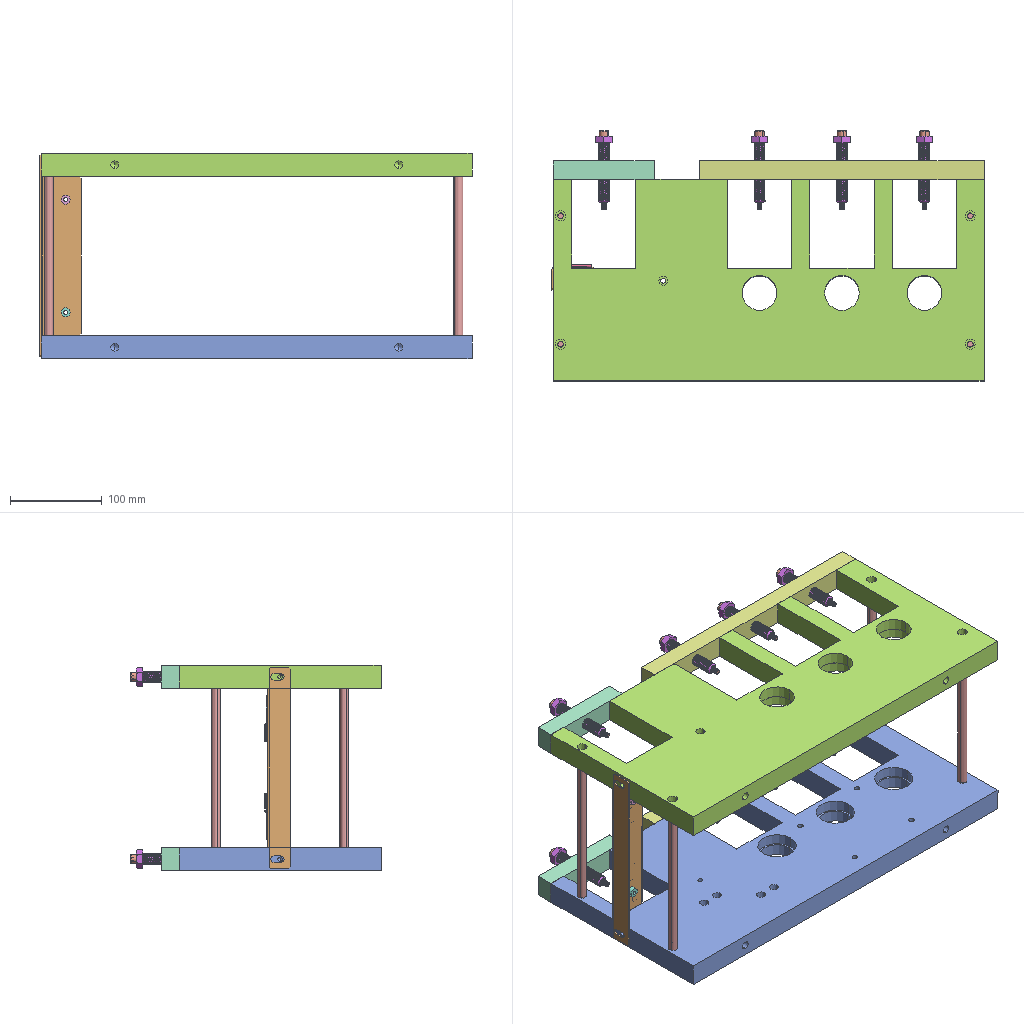Assembly | SolidWorks | 9 different items | 29 placed | box 472 x 273 x 224 mm
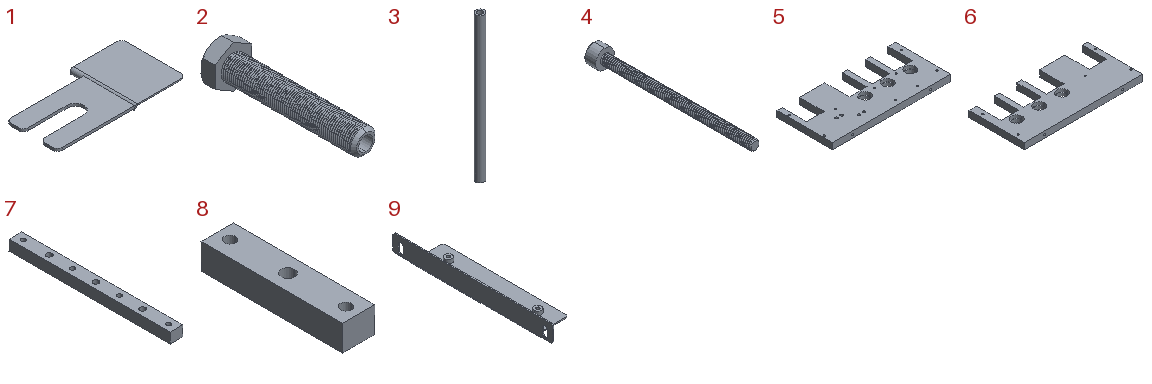Parts list (item | quantity | size | volume | features):
1 | x2 | 50 x 25 x 2.5 mm | 876.083 mm3 | features ICE 4, Fillet 2, FlatPattern 2, SMBaseFlange 2, SheetMetal 2, MirrorSolid 1
2 | x8 | 18 x 71.9 x 20.785 mm | 5747 mm3 | features ICE 2, Chamfer 1, Extrusion 1, RevCut 1, SweepThread 1
3 | x4 | 10 x 10 x 174 mm | 13100 mm3 | features Extrusion 1, ICE 1, MirrorPattern 1
4 | x8 | 10 x 86 x 10 mm | 1649 mm3 | features ICE 2, Chamfer 1, Extrusion 1, Fillet 1, SweepThread 1
5 | x1 | 470 x 220 x 25 mm | 1786055 mm3 | features ICE 8, HoleWzd 3, Cut 2, 3DProfileFeature 1, Extrusion 1, LPattern 1
6 | x1 | 470 x 220 x 25 mm | 1796756 mm3 | features ICE 8, HoleWzd 3, LPattern 2, 3DProfileFeature 1, Extrusion 1
7 | x2 | 25 x 310 x 20 mm | 142225 mm3 | features ICE 2, Extrusion 1, HoleWzd 1
8 | x2 | 25 x 110 x 20 mm | 49479 mm3 | features ICE 2, Extrusion 1, HoleWzd 1
9 | x1 | 45 x 220 x 25 mm | 19511 mm3 | features ICE 3, HoleWzd 2, Chamfer 1, FlatPattern 1, SMBaseFlange 1, SheetMetal 1
Mates (type | each side: item.copy, entity, surface, feature):
Coincident | 6.1 face plane Boss-Extrude1 | 3.1 face plane Boss-Extrude1
Concentric | 6.1 face cylinder Cut-Extrude9 | 3.1 face cylinder Boss-Extrude1
Coincident | 5.1 face plane Boss-Extrude1 | 6.1 face plane Boss-Extrude1
Coincident | 5.1 face plane Cut-Extrude7 | 6.1 face plane Cut-Extrude6
DistanceDim | 6.1 face plane Boss-Extrude1 | 5.1 face plane Boss-Extrude1
Coincident | 9.1 face plane Base-Flange1 | 1.1 face plane Base-Flange2
Coincident | 9.1 face plane Base-Flange1 | 1.2 face plane Mirror1
Coincident | 6.1 face plane Boss-Extrude1 | 9.1 face plane Base-Flange1
Width | 9.1 face plane Cut-Extrude2 | 9.1 face plane Cut-Extrude2 | 6.1 face cylinder M6 Tapped Hole1
Coincident | 1.2 face plane Mirror1 | 1.1 face plane Base-Flange1
Parallel | 5.1 face plane Boss-Extrude1 | 1.2 face plane Mirror1
Coincident | 5.1 face plane Boss-Extrude1 | 7.1 face plane Boss-Extrude1 | 3 times
Concentric | 7.1 face cylinder M12x1.25 Tapped Hole1 | 2.1 face cone Chamfer1
Coincident | 5.1 face plane Boss-Extrude1 | 8.1 face plane Boss-Extrude1 | 3 times
Concentric | 8.1 face cylinder M12x1.25 Tapped Hole1 | 2.2 face cone Chamfer1
Concentric | 2.3 face cylinder Cut-Extrude1 | 4.1 face cylinder Boss-Extrude1
Coincident | 2.3 face plane Boss-Extrude1 | 4.1 face plane Boss-Extrude1
Concentric | 7.1 face cylinder M12x1.25 Tapped Hole1 | 2.3 face cone Chamfer1
Concentric | 2.1 face cylinder Cut-Extrude1 | 4.2 face cylinder Boss-Extrude1
Coincident | 2.1 face plane Boss-Extrude1 | 4.2 face plane Boss-Extrude1
Concentric | 2.4 face cylinder Cut-Extrude1 | 4.3 face cylinder Boss-Extrude1
Coincident | 2.4 face plane Boss-Extrude1 | 4.3 face plane Boss-Extrude1
Concentric | 7.1 face cylinder M12x1.25 Tapped Hole1 | 2.4 face cone Chamfer1
Concentric | 2.2 face cylinder Cut-Extrude1 | 4.4 face cylinder Boss-Extrude1
Coincident | 2.2 face plane Boss-Extrude1 | 4.4 face plane Boss-Extrude1